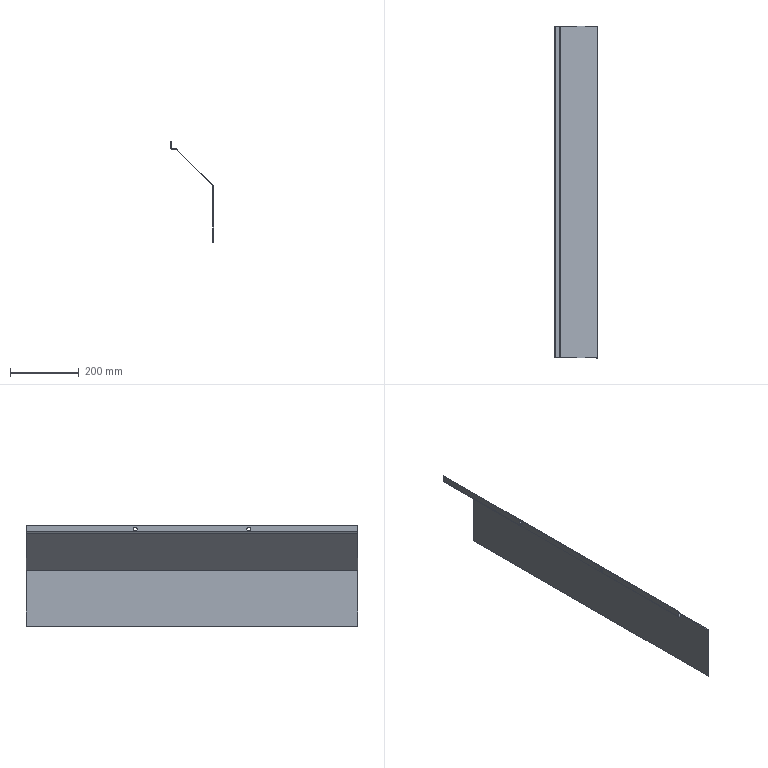Part | STEP file | SYL_0392D6J1SYL0380DJ10-1577336 | 1 solid | 38 faces | box 125 x 964 x 292 mm | volume 507408 mm3 | plane 28 | cylinder 10 | commonest cylinder face diameters 8 x4 4 x3 7 x3
STEP:
#1=CARTESIAN_POINT('',(0.,163.,6.));
#2=VERTEX_POINT('',#1);
#3=CARTESIAN_POINT('',(-1.5,163.,6.));
#4=VERTEX_POINT('',#3);
#5=CARTESIAN_POINT('',(-1.5,163.,6.));
#6=DIRECTION('',(-1.,0.,0.));
#7=VECTOR('',#6,1000.);
#8=LINE('',#5,#7);
#9=EDGE_CURVE('',#2,#4,#8,.T.);
#10=ORIENTED_EDGE('',*,*,#9,.F.);
#11=CARTESIAN_POINT('',(0.,167.,6.));
#12=VERTEX_POINT('',#11);
#13=CARTESIAN_POINT('',(0.,-482.,6.));
#14=DIRECTION('',(0.,1.,0.));
#15=VECTOR('',#14,1000.);
#16=LINE('',#13,#15);
#17=EDGE_CURVE('',#2,#12,#16,.T.);
#18=ORIENTED_EDGE('',*,*,#17,.T.);
#19=CARTESIAN_POINT('',(-1.5,167.,6.));
#20=VERTEX_POINT('',#19);
#21=CARTESIAN_POINT('',(-1.5,167.,6.));
#22=DIRECTION('',(-1.,0.,0.));
#23=VECTOR('',#22,1000.);
#24=LINE('',#21,#23);
#25=EDGE_CURVE('',#12,#20,#24,.T.);
#26=ORIENTED_EDGE('',*,*,#25,.T.);
#27=CARTESIAN_POINT('',(-1.5,163.,6.));
#28=DIRECTION('',(0.,1.,0.));
#29=VECTOR('',#28,1000.);
#30=LINE('',#27,#29);
#31=EDGE_CURVE('',#4,#20,#30,.T.);
#32=ORIENTED_EDGE('',*,*,#31,.F.);
#33=EDGE_LOOP('',(#10,#18,#26,#32));
#34=FACE_OUTER_BOUND('',#33,.T.);
#35=CARTESIAN_POINT('',(-1.5,163.,6.));
#36=DIRECTION('',(0.,0.,-1.));
#37=DIRECTION('',(0.,1.,0.));
#38=AXIS2_PLACEMENT_3D('',#35,#36,#37);
#39=PLANE('',#38);
#40=ADVANCED_FACE('',(#34),#39,.F.);
#41=ORIENTED_EDGE('',*,*,#25,.F.);
#42=CARTESIAN_POINT('',(0.,167.,14.));
#43=VERTEX_POINT('',#42);
#44=CARTESIAN_POINT('',(0.,167.,10.));
#45=DIRECTION('',(1.,0.,0.));
#46=DIRECTION('',(0.,0.,-1.));
#47=AXIS2_PLACEMENT_3D('',#44,#45,#46);
#48=CIRCLE('',#47,4.);
#49=EDGE_CURVE('',#12,#43,#48,.T.);
#50=ORIENTED_EDGE('',*,*,#49,.T.);
#51=CARTESIAN_POINT('',(-1.5,167.,14.));
#52=VERTEX_POINT('',#51);
#53=CARTESIAN_POINT('',(-1.5,167.,14.));
#54=DIRECTION('',(-1.,0.,0.));
#55=VECTOR('',#54,1000.);
#56=LINE('',#53,#55);
#57=EDGE_CURVE('',#43,#52,#56,.T.);
#58=ORIENTED_EDGE('',*,*,#57,.T.);
#59=CARTESIAN_POINT('',(-1.5,167.,10.));
#60=DIRECTION('',(1.,0.,0.));
#61=DIRECTION('',(0.,0.,-1.));
#62=AXIS2_PLACEMENT_3D('',#59,#60,#61);
#63=CIRCLE('',#62,4.);
#64=EDGE_CURVE('',#20,#52,#63,.T.);
#65=ORIENTED_EDGE('',*,*,#64,.F.);
#66=EDGE_LOOP('',(#41,#50,#58,#65));
#67=FACE_OUTER_BOUND('',#66,.T.);
#68=CARTESIAN_POINT('',(-1.5,167.,10.));
#69=DIRECTION('',(1.,0.,0.));
#70=DIRECTION('',(0.,0.,-1.));
#71=AXIS2_PLACEMENT_3D('',#68,#69,#70);
#72=CYLINDRICAL_SURFACE('',#71,4.);
#73=ADVANCED_FACE('',(#67),#72,.F.);
#74=ORIENTED_EDGE('',*,*,#57,.F.);
#75=CARTESIAN_POINT('',(0.,163.,14.));
#76=VERTEX_POINT('',#75);
#77=CARTESIAN_POINT('',(0.,-482.,14.));
#78=DIRECTION('',(0.,-1.,0.));
#79=VECTOR('',#78,1000.);
#80=LINE('',#77,#79);
#81=EDGE_CURVE('',#43,#76,#80,.T.);
#82=ORIENTED_EDGE('',*,*,#81,.T.);
#83=CARTESIAN_POINT('',(-1.5,163.,14.));
#84=VERTEX_POINT('',#83);
#85=CARTESIAN_POINT('',(-1.5,163.,14.));
#86=DIRECTION('',(-1.,0.,0.));
#87=VECTOR('',#86,1000.);
#88=LINE('',#85,#87);
#89=EDGE_CURVE('',#76,#84,#88,.T.);
#90=ORIENTED_EDGE('',*,*,#89,.T.);
#91=CARTESIAN_POINT('',(-1.5,167.,14.));
#92=DIRECTION('',(0.,-1.,0.));
#93=VECTOR('',#92,1000.);
#94=LINE('',#91,#93);
#95=EDGE_CURVE('',#52,#84,#94,.T.);
#96=ORIENTED_EDGE('',*,*,#95,.F.);
#97=EDGE_LOOP('',(#74,#82,#90,#96));
#98=FACE_OUTER_BOUND('',#97,.T.);
#99=CARTESIAN_POINT('',(-1.5,167.,14.));
#100=DIRECTION('',(0.,0.,1.));
#101=DIRECTION('',(0.,-1.,0.));
#102=AXIS2_PLACEMENT_3D('',#99,#100,#101);
#103=PLANE('',#102);
#104=ADVANCED_FACE('',(#98),#103,.F.);
#105=CARTESIAN_POINT('',(0.,-163.,6.));
#106=VERTEX_POINT('',#105);
#107=CARTESIAN_POINT('',(-1.5,-163.,6.));
#108=VERTEX_POINT('',#107);
#109=CARTESIAN_POINT('',(-1.5,-163.,6.));
#110=DIRECTION('',(-1.,0.,0.));
#111=VECTOR('',#110,1000.);
#112=LINE('',#109,#111);
#113=EDGE_CURVE('',#106,#108,#112,.T.);
#114=ORIENTED_EDGE('',*,*,#113,.F.);
#115=CARTESIAN_POINT('',(0.,-163.,14.));
#116=VERTEX_POINT('',#115);
#117=CARTESIAN_POINT('',(0.,-163.,10.));
#118=DIRECTION('',(1.,0.,0.));
#119=DIRECTION('',(0.,0.,-1.));
#120=AXIS2_PLACEMENT_3D('',#117,#118,#119);
#121=CIRCLE('',#120,4.);
#122=EDGE_CURVE('',#106,#116,#121,.T.);
#123=ORIENTED_EDGE('',*,*,#122,.T.);
#124=CARTESIAN_POINT('',(-1.5,-163.,14.));
#125=VERTEX_POINT('',#124);
#126=CARTESIAN_POINT('',(-1.5,-163.,14.));
#127=DIRECTION('',(-1.,0.,0.));
#128=VECTOR('',#127,1000.);
#129=LINE('',#126,#128);
#130=EDGE_CURVE('',#116,#125,#129,.T.);
#131=ORIENTED_EDGE('',*,*,#130,.T.);
#132=CARTESIAN_POINT('',(-1.5,-163.,10.));
#133=DIRECTION('',(1.,0.,0.));
#134=DIRECTION('',(0.,0.,-1.));
#135=AXIS2_PLACEMENT_3D('',#132,#133,#134);
#136=CIRCLE('',#135,4.);
#137=EDGE_CURVE('',#108,#125,#136,.T.);
#138=ORIENTED_EDGE('',*,*,#137,.F.);
#139=EDGE_LOOP('',(#114,#123,#131,#138));
#140=FACE_OUTER_BOUND('',#139,.T.);
#141=CARTESIAN_POINT('',(-1.5,-163.,10.));
#142=DIRECTION('',(1.,0.,0.));
#143=DIRECTION('',(0.,0.,-1.));
#144=AXIS2_PLACEMENT_3D('',#141,#142,#143);
#145=CYLINDRICAL_SURFACE('',#144,4.);
#146=ADVANCED_FACE('',(#140),#145,.F.);
#147=ORIENTED_EDGE('',*,*,#130,.F.);
#148=CARTESIAN_POINT('',(0.,-167.,14.));
#149=VERTEX_POINT('',#148);
#150=CARTESIAN_POINT('',(0.,-482.,14.));
#151=DIRECTION('',(0.,-1.,0.));
#152=VECTOR('',#151,1000.);
#153=LINE('',#150,#152);
#154=EDGE_CURVE('',#116,#149,#153,.T.);
#155=ORIENTED_EDGE('',*,*,#154,.T.);
#156=CARTESIAN_POINT('',(-1.5,-167.,14.));
#157=VERTEX_POINT('',#156);
#158=CARTESIAN_POINT('',(-1.5,-167.,14.));
#159=DIRECTION('',(-1.,0.,0.));
#160=VECTOR('',#159,1000.);
#161=LINE('',#158,#160);
#162=EDGE_CURVE('',#149,#157,#161,.T.);
#163=ORIENTED_EDGE('',*,*,#162,.T.);
#164=CARTESIAN_POINT('',(-1.5,-163.,14.));
#165=DIRECTION('',(0.,-1.,0.));
#166=VECTOR('',#165,1000.);
#167=LINE('',#164,#166);
#168=EDGE_CURVE('',#125,#157,#167,.T.);
#169=ORIENTED_EDGE('',*,*,#168,.F.);
#170=EDGE_LOOP('',(#147,#155,#163,#169));
#171=FACE_OUTER_BOUND('',#170,.T.);
#172=CARTESIAN_POINT('',(-1.5,-163.,14.));
#173=DIRECTION('',(0.,0.,1.));
#174=DIRECTION('',(0.,-1.,0.));
#175=AXIS2_PLACEMENT_3D('',#172,#173,#174);
#176=PLANE('',#175);
#177=ADVANCED_FACE('',(#171),#176,.F.);
#178=ORIENTED_EDGE('',*,*,#162,.F.);
#179=CARTESIAN_POINT('',(0.,-167.,6.));
#180=VERTEX_POINT('',#179);
#181=CARTESIAN_POINT('',(0.,-167.,10.));
#182=DIRECTION('',(1.,0.,0.));
#183=DIRECTION('',(0.,0.,-1.));
#184=AXIS2_PLACEMENT_3D('',#181,#182,#183);
#185=CIRCLE('',#184,4.);
#186=EDGE_CURVE('',#149,#180,#185,.T.);
#187=ORIENTED_EDGE('',*,*,#186,.T.);
#188=CARTESIAN_POINT('',(-1.5,-167.,6.));
#189=VERTEX_POINT('',#188);
#190=CARTESIAN_POINT('',(-1.5,-167.,6.));
#191=DIRECTION('',(-1.,0.,0.));
#192=VECTOR('',#191,1000.);
#193=LINE('',#190,#192);
#194=EDGE_CURVE('',#180,#189,#193,.T.);
#195=ORIENTED_EDGE('',*,*,#194,.T.);
#196=CARTESIAN_POINT('',(-1.5,-167.,10.));
#197=DIRECTION('',(1.,0.,0.));
#198=DIRECTION('',(0.,0.,1.));
#199=AXIS2_PLACEMENT_3D('',#196,#197,#198);
#200=CIRCLE('',#199,4.);
#201=EDGE_CURVE('',#157,#189,#200,.T.);
#202=ORIENTED_EDGE('',*,*,#201,.F.);
#203=EDGE_LOOP('',(#178,#187,#195,#202));
#204=FACE_OUTER_BOUND('',#203,.T.);
#205=CARTESIAN_POINT('',(-1.5,-167.,10.));
#206=DIRECTION('',(1.,0.,0.));
#207=DIRECTION('',(0.,0.,-1.));
#208=AXIS2_PLACEMENT_3D('',#205,#206,#207);
#209=CYLINDRICAL_SURFACE('',#208,4.);
#210=ADVANCED_FACE('',(#204),#209,.F.);
#211=CARTESIAN_POINT('',(0.,-482.,20.));
#212=VERTEX_POINT('',#211);
#213=CARTESIAN_POINT('',(-1.5,-482.,20.));
#214=VERTEX_POINT('',#213);
#215=CARTESIAN_POINT('',(-1.5,-482.,20.));
#216=DIRECTION('',(-1.,0.,0.));
#217=VECTOR('',#216,1000.);
#218=LINE('',#215,#217);
#219=EDGE_CURVE('',#212,#214,#218,.T.);
#220=ORIENTED_EDGE('',*,*,#219,.F.);
#221=CARTESIAN_POINT('',(0.,482.,20.));
#222=VERTEX_POINT('',#221);
#223=CARTESIAN_POINT('',(0.,-482.,20.));
#224=DIRECTION('',(0.,-1.,0.));
#225=VECTOR('',#224,1000.);
#226=LINE('',#223,#225);
#227=EDGE_CURVE('',#222,#212,#226,.T.);
#228=ORIENTED_EDGE('',*,*,#227,.F.);
#229=CARTESIAN_POINT('',(-1.5,482.,20.));
#230=VERTEX_POINT('',#229);
#231=CARTESIAN_POINT('',(-1.5,482.,20.));
#232=DIRECTION('',(-1.,0.,0.));
#233=VECTOR('',#232,1000.);
#234=LINE('',#231,#233);
#235=EDGE_CURVE('',#222,#230,#234,.T.);
#236=ORIENTED_EDGE('',*,*,#235,.T.);
#237=CARTESIAN_POINT('',(-1.5,482.,20.));
#238=DIRECTION('',(0.,-1.,0.));
#239=VECTOR('',#238,1000.);
#240=LINE('',#237,#239);
#241=EDGE_CURVE('',#230,#214,#240,.T.);
#242=ORIENTED_EDGE('',*,*,#241,.T.);
#243=EDGE_LOOP('',(#220,#228,#236,#242));
#244=FACE_OUTER_BOUND('',#243,.T.);
#245=CARTESIAN_POINT('',(-1.5,482.,20.));
#246=DIRECTION('',(0.,0.,1.));
#247=DIRECTION('',(0.,-1.,0.));
#248=AXIS2_PLACEMENT_3D('',#245,#246,#247);
#249=PLANE('',#248);
#250=ADVANCED_FACE('',(#244),#249,.T.);
#251=ORIENTED_EDGE('',*,*,#235,.F.);
#252=CARTESIAN_POINT('',(0.,482.,2.));
#253=VERTEX_POINT('',#252);
#254=CARTESIAN_POINT('',(0.,482.,20.));
#255=DIRECTION('',(0.,0.,1.));
#256=VECTOR('',#255,1000.);
#257=LINE('',#254,#256);
#258=EDGE_CURVE('',#253,#222,#257,.T.);
#259=ORIENTED_EDGE('',*,*,#258,.F.);
#260=CARTESIAN_POINT('',(-1.5,482.,2.));
#261=VERTEX_POINT('',#260);
#262=CARTESIAN_POINT('',(-1.5,482.,2.));
#263=DIRECTION('',(-1.,0.,0.));
#264=VECTOR('',#263,1000.);
#265=LINE('',#262,#264);
#266=EDGE_CURVE('',#253,#261,#265,.T.);
#267=ORIENTED_EDGE('',*,*,#266,.T.);
#268=CARTESIAN_POINT('',(-1.5,482.,2.));
#269=DIRECTION('',(0.,0.,1.));
#270=VECTOR('',#269,1000.);
#271=LINE('',#268,#270);
#272=EDGE_CURVE('',#261,#230,#271,.T.);
#273=ORIENTED_EDGE('',*,*,#272,.T.);
#274=EDGE_LOOP('',(#251,#259,#267,#273));
#275=FACE_OUTER_BOUND('',#274,.T.);
#276=CARTESIAN_POINT('',(-1.5,482.,2.));
#277=DIRECTION('',(0.,1.,0.));
#278=DIRECTION('',(0.,0.,1.));
#279=AXIS2_PLACEMENT_3D('',#276,#277,#278);
#280=PLANE('',#279);
#281=ADVANCED_FACE('',(#275),#280,.T.);
#282=ORIENTED_EDGE('',*,*,#266,.F.);
#283=CARTESIAN_POINT('',(2.,482.,0.));
#284=VERTEX_POINT('',#283);
#285=CARTESIAN_POINT('',(2.,482.,2.));
#286=DIRECTION('',(0.,1.,0.));
#287=DIRECTION('',(0.,0.,1.));
#288=AXIS2_PLACEMENT_3D('',#285,#286,#287);
#289=CIRCLE('',#288,2.);
#290=EDGE_CURVE('',#284,#253,#289,.T.);
#291=ORIENTED_EDGE('',*,*,#290,.F.);
#292=CARTESIAN_POINT('',(2.,482.,-1.5));
#293=VERTEX_POINT('',#292);
#294=CARTESIAN_POINT('',(2.,482.,-1.5));
#295=DIRECTION('',(0.,0.,-1.));
#296=VECTOR('',#295,1000.);
#297=LINE('',#294,#296);
#298=EDGE_CURVE('',#284,#293,#297,.T.);
#299=ORIENTED_EDGE('',*,*,#298,.T.);
#300=CARTESIAN_POINT('',(2.,482.,2.));
#301=DIRECTION('',(0.,1.,0.));
#302=DIRECTION('',(0.,0.,-1.));
#303=AXIS2_PLACEMENT_3D('',#300,#301,#302);
#304=CIRCLE('',#303,3.5);
#305=EDGE_CURVE('',#293,#261,#304,.T.);
#306=ORIENTED_EDGE('',*,*,#305,.T.);
#307=EDGE_LOOP('',(#282,#291,#299,#306));
#308=FACE_OUTER_BOUND('',#307,.T.);
#309=CARTESIAN_POINT('',(2.,482.,2.));
#310=DIRECTION('',(0.,-1.,0.));
#311=DIRECTION('',(0.,0.,-1.));
#312=AXIS2_PLACEMENT_3D('',#309,#310,#311);
#313=PLANE('',#312);
#314=ADVANCED_FACE('',(#308),#313,.F.);
#315=ORIENTED_EDGE('',*,*,#298,.F.);
#316=CARTESIAN_POINT('',(14.05,482.,0.));
#317=VERTEX_POINT('',#316);
#318=CARTESIAN_POINT('',(0.,482.,0.));
#319=DIRECTION('',(-1.,0.,0.));
#320=VECTOR('',#319,1000.);
#321=LINE('',#318,#320);
#322=EDGE_CURVE('',#317,#284,#321,.T.);
#323=ORIENTED_EDGE('',*,*,#322,.F.);
#324=CARTESIAN_POINT('',(14.05,482.,-1.5));
#325=VERTEX_POINT('',#324);
#326=CARTESIAN_POINT('',(14.05,482.,-1.5));
#327=DIRECTION('',(0.,0.,-1.));
#328=VECTOR('',#327,1000.);
#329=LINE('',#326,#328);
#330=EDGE_CURVE('',#317,#325,#329,.T.);
#331=ORIENTED_EDGE('',*,*,#330,.T.);
#332=CARTESIAN_POINT('',(14.05,482.,-1.5));
#333=DIRECTION('',(-1.,0.,0.));
#334=VECTOR('',#333,1000.);
#335=LINE('',#332,#334);
#336=EDGE_CURVE('',#325,#293,#335,.T.);
#337=ORIENTED_EDGE('',*,*,#336,.T.);
#338=EDGE_LOOP('',(#315,#323,#331,#337));
#339=FACE_OUTER_BOUND('',#338,.T.);
#340=CARTESIAN_POINT('',(14.05,482.,-1.5));
#341=DIRECTION('',(0.,1.,0.));
#342=DIRECTION('',(-1.,0.,0.));
#343=AXIS2_PLACEMENT_3D('',#340,#341,#342);
#344=PLANE('',#343);
#345=ADVANCED_FACE('',(#339),#344,.T.);
#346=ORIENTED_EDGE('',*,*,#330,.F.);
#347=CARTESIAN_POINT('',(16.525,482.,-1.025));
#348=VERTEX_POINT('',#347);
#349=CARTESIAN_POINT('',(14.05,482.,-3.5));
#350=DIRECTION('',(0.,-1.,0.));
#351=DIRECTION('',(0.,0.,-1.));
#352=AXIS2_PLACEMENT_3D('',#349,#350,#351);
#353=CIRCLE('',#352,3.5);
#354=EDGE_CURVE('',#348,#317,#353,.T.);
#355=ORIENTED_EDGE('',*,*,#354,.F.);
#356=CARTESIAN_POINT('',(15.464,482.,-2.086));
#357=VERTEX_POINT('',#356);
#358=CARTESIAN_POINT('',(15.464,482.,-2.086));
#359=DIRECTION('',(-0.7071,0.,-0.7071));
#360=VECTOR('',#359,1000.);
#361=LINE('',#358,#360);
#362=EDGE_CURVE('',#348,#357,#361,.T.);
#363=ORIENTED_EDGE('',*,*,#362,.T.);
#364=CARTESIAN_POINT('',(14.05,482.,-3.5));
#365=DIRECTION('',(0.,-1.,0.));
#366=DIRECTION('',(0.7071,0.,0.7071));
#367=AXIS2_PLACEMENT_3D('',#364,#365,#366);
#368=CIRCLE('',#367,2.);
#369=EDGE_CURVE('',#357,#325,#368,.T.);
#370=ORIENTED_EDGE('',*,*,#369,.T.);
#371=EDGE_LOOP('',(#346,#355,#363,#370));
#372=FACE_OUTER_BOUND('',#371,.T.);
#373=CARTESIAN_POINT('',(14.05,482.,-3.5));
#374=DIRECTION('',(0.,1.,0.));
#375=DIRECTION('',(0.,0.,1.));
#376=AXIS2_PLACEMENT_3D('',#373,#374,#375);
#377=PLANE('',#376);
#378=ADVANCED_FACE('',(#372),#377,.T.);
#379=ORIENTED_EDGE('',*,*,#362,.F.);
#380=CARTESIAN_POINT('',(122.475,482.,-106.975));
#381=VERTEX_POINT('',#380);
#382=CARTESIAN_POINT('',(15.5,482.,0.));
#383=DIRECTION('',(-0.7071,0.,0.7071));
#384=VECTOR('',#383,1000.);
#385=LINE('',#382,#384);
#386=EDGE_CURVE('',#381,#348,#385,.T.);
#387=ORIENTED_EDGE('',*,*,#386,.F.);
#388=CARTESIAN_POINT('',(121.414,482.,-108.036));
#389=VERTEX_POINT('',#388);
#390=CARTESIAN_POINT('',(121.414,482.,-108.036));
#391=DIRECTION('',(-0.7071,0.,-0.7071));
#392=VECTOR('',#391,1000.);
#393=LINE('',#390,#392);
#394=EDGE_CURVE('',#381,#389,#393,.T.);
#395=ORIENTED_EDGE('',*,*,#394,.T.);
#396=CARTESIAN_POINT('',(121.414,482.,-108.036));
#397=DIRECTION('',(-0.7071,0.,0.7071));
#398=VECTOR('',#397,1000.);
#399=LINE('',#396,#398);
#400=EDGE_CURVE('',#389,#357,#399,.T.);
#401=ORIENTED_EDGE('',*,*,#400,.T.);
#402=EDGE_LOOP('',(#379,#387,#395,#401));
#403=FACE_OUTER_BOUND('',#402,.T.);
#404=CARTESIAN_POINT('',(121.414,482.,-108.036));
#405=DIRECTION('',(0.,1.,0.));
#406=DIRECTION('',(-0.7071,0.,0.7071));
#407=AXIS2_PLACEMENT_3D('',#404,#405,#406);
#408=PLANE('',#407);
#409=ADVANCED_FACE('',(#403),#408,.T.);
#410=ORIENTED_EDGE('',*,*,#394,.F.);
#411=CARTESIAN_POINT('',(123.5,482.,-109.45));
#412=VERTEX_POINT('',#411);
#413=CARTESIAN_POINT('',(120.,482.,-109.45));
#414=DIRECTION('',(0.,-1.,0.));
#415=DIRECTION('',(0.,0.,-1.));
#416=AXIS2_PLACEMENT_3D('',#413,#414,#415);
#417=CIRCLE('',#416,3.5);
#418=EDGE_CURVE('',#412,#381,#417,.T.);
#419=ORIENTED_EDGE('',*,*,#418,.F.);
#420=CARTESIAN_POINT('',(122.,482.,-109.45));
#421=VERTEX_POINT('',#420);
#422=CARTESIAN_POINT('',(122.,482.,-109.45));
#423=DIRECTION('',(-1.,0.,0.));
#424=VECTOR('',#423,1000.);
#425=LINE('',#422,#424);
#426=EDGE_CURVE('',#412,#421,#425,.T.);
#427=ORIENTED_EDGE('',*,*,#426,.T.);
#428=CARTESIAN_POINT('',(120.,482.,-109.45));
#429=DIRECTION('',(0.,-1.,0.));
#430=DIRECTION('',(1.,0.,0.));
#431=AXIS2_PLACEMENT_3D('',#428,#429,#430);
#432=CIRCLE('',#431,2.);
#433=EDGE_CURVE('',#421,#389,#432,.T.);
#434=ORIENTED_EDGE('',*,*,#433,.T.);
#435=EDGE_LOOP('',(#410,#419,#427,#434));
#436=FACE_OUTER_BOUND('',#435,.T.);
#437=CARTESIAN_POINT('',(120.,482.,-109.45));
#438=DIRECTION('',(0.,1.,0.));
#439=DIRECTION('',(0.,0.,1.));
#440=AXIS2_PLACEMENT_3D('',#437,#438,#439);
#441=PLANE('',#440);
#442=ADVANCED_FACE('',(#436),#441,.T.);
#443=ORIENTED_EDGE('',*,*,#426,.F.);
#444=CARTESIAN_POINT('',(123.5,482.,-272.));
#445=VERTEX_POINT('',#444);
#446=CARTESIAN_POINT('',(123.5,482.,-108.));
#447=DIRECTION('',(0.,0.,1.));
#448=VECTOR('',#447,1000.);
#449=LINE('',#446,#448);
#450=EDGE_CURVE('',#445,#412,#449,.T.);
#451=ORIENTED_EDGE('',*,*,#450,.F.);
#452=CARTESIAN_POINT('',(122.,482.,-272.));
#453=VERTEX_POINT('',#452);
#454=CARTESIAN_POINT('',(122.,482.,-272.));
#455=DIRECTION('',(-1.,0.,0.));
#456=VECTOR('',#455,1000.);
#457=LINE('',#454,#456);
#458=EDGE_CURVE('',#445,#453,#457,.T.);
#459=ORIENTED_EDGE('',*,*,#458,.T.);
#460=CARTESIAN_POINT('',(122.,482.,-272.));
#461=DIRECTION('',(0.,0.,1.));
#462=VECTOR('',#461,1000.);
#463=LINE('',#460,#462);
#464=EDGE_CURVE('',#453,#421,#463,.T.);
#465=ORIENTED_EDGE('',*,*,#464,.T.);
#466=EDGE_LOOP('',(#443,#451,#459,#465));
#467=FACE_OUTER_BOUND('',#466,.T.);
#468=CARTESIAN_POINT('',(122.,482.,-272.));
#469=DIRECTION('',(0.,1.,0.));
#470=DIRECTION('',(0.,0.,1.));
#471=AXIS2_PLACEMENT_3D('',#468,#469,#470);
#472=PLANE('',#471);
#473=ADVANCED_FACE('',(#467),#472,.T.);
#474=ORIENTED_EDGE('',*,*,#458,.F.);
#475=CARTESIAN_POINT('',(123.5,-482.,-272.));
#476=VERTEX_POINT('',#475);
#477=CARTESIAN_POINT('',(123.5,-482.,-272.));
#478=DIRECTION('',(0.,-1.,0.));
#479=VECTOR('',#478,1000.);
#480=LINE('',#477,#479);
#481=EDGE_CURVE('',#445,#476,#480,.T.);
#482=ORIENTED_EDGE('',*,*,#481,.T.);
#483=CARTESIAN_POINT('',(122.,-482.,-272.));
#484=VERTEX_POINT('',#483);
#485=CARTESIAN_POINT('',(122.,-482.,-272.));
#486=DIRECTION('',(-1.,0.,0.));
#487=VECTOR('',#486,1000.);
#488=LINE('',#485,#487);
#489=EDGE_CURVE('',#476,#484,#488,.T.);
#490=ORIENTED_EDGE('',*,*,#489,.T.);
#491=CARTESIAN_POINT('',(122.,482.,-272.));
#492=DIRECTION('',(0.,-1.,0.));
#493=VECTOR('',#492,1000.);
#494=LINE('',#491,#493);
#495=EDGE_CURVE('',#453,#484,#494,.T.);
#496=ORIENTED_EDGE('',*,*,#495,.F.);
#497=EDGE_LOOP('',(#474,#482,#490,#496));
#498=FACE_OUTER_BOUND('',#497,.T.);
#499=CARTESIAN_POINT('',(122.,482.,-272.));
#500=DIRECTION('',(0.,0.,1.));
#501=DIRECTION('',(0.,-1.,0.));
#502=AXIS2_PLACEMENT_3D('',#499,#500,#501);
#503=PLANE('',#502);
#504=ADVANCED_FACE('',(#498),#503,.F.);
#505=ORIENTED_EDGE('',*,*,#489,.F.);
#506=CARTESIAN_POINT('',(123.5,-482.,-109.45));
#507=VERTEX_POINT('',#506);
#508=CARTESIAN_POINT('',(123.5,-482.,-108.));
#509=DIRECTION('',(0.,0.,1.));
#510=VECTOR('',#509,1000.);
#511=LINE('',#508,#510);
#512=EDGE_CURVE('',#476,#507,#511,.T.);
#513=ORIENTED_EDGE('',*,*,#512,.T.);
#514=CARTESIAN_POINT('',(122.,-482.,-109.45));
#515=VERTEX_POINT('',#514);
#516=CARTESIAN_POINT('',(122.,-482.,-109.45));
#517=DIRECTION('',(-1.,0.,0.));
#518=VECTOR('',#517,1000.);
#519=LINE('',#516,#518);
#520=EDGE_CURVE('',#507,#515,#519,.T.);
#521=ORIENTED_EDGE('',*,*,#520,.T.);
#522=CARTESIAN_POINT('',(122.,-482.,-272.));
#523=DIRECTION('',(0.,0.,1.));
#524=VECTOR('',#523,1000.);
#525=LINE('',#522,#524);
#526=EDGE_CURVE('',#484,#515,#525,.T.);
#527=ORIENTED_EDGE('',*,*,#526,.F.);
#528=EDGE_LOOP('',(#505,#513,#521,#527));
#529=FACE_OUTER_BOUND('',#528,.T.);
#530=CARTESIAN_POINT('',(122.,-482.,-272.));
#531=DIRECTION('',(0.,1.,0.));
#532=DIRECTION('',(0.,0.,1.));
#533=AXIS2_PLACEMENT_3D('',#530,#531,#532);
#534=PLANE('',#533);
#535=ADVANCED_FACE('',(#529),#534,.F.);
#536=ORIENTED_EDGE('',*,*,#520,.F.);
#537=CARTESIAN_POINT('',(122.475,-482.,-106.975));
#538=VERTEX_POINT('',#537);
#539=CARTESIAN_POINT('',(120.,-482.,-109.45));
#540=DIRECTION('',(0.,1.,0.));
#541=DIRECTION('',(0.,0.,-1.));
#542=AXIS2_PLACEMENT_3D('',#539,#540,#541);
#543=CIRCLE('',#542,3.5);
#544=EDGE_CURVE('',#538,#507,#543,.T.);
#545=ORIENTED_EDGE('',*,*,#544,.F.);
#546=CARTESIAN_POINT('',(121.414,-482.,-108.036));
#547=VERTEX_POINT('',#546);
#548=CARTESIAN_POINT('',(121.414,-482.,-108.036));
#549=DIRECTION('',(-0.7071,0.,-0.7071));
#550=VECTOR('',#549,1000.);
#551=LINE('',#548,#550);
#552=EDGE_CURVE('',#538,#547,#551,.T.);
#553=ORIENTED_EDGE('',*,*,#552,.T.);
#554=CARTESIAN_POINT('',(120.,-482.,-109.45));
#555=DIRECTION('',(0.,1.,0.));
#556=DIRECTION('',(0.7071,0.,0.7071));
#557=AXIS2_PLACEMENT_3D('',#554,#555,#556);
#558=CIRCLE('',#557,2.);
#559=EDGE_CURVE('',#547,#515,#558,.T.);
#560=ORIENTED_EDGE('',*,*,#559,.T.);
#561=EDGE_LOOP('',(#536,#545,#553,#560));
#562=FACE_OUTER_BOUND('',#561,.T.);
#563=CARTESIAN_POINT('',(120.,-482.,-109.45));
#564=DIRECTION('',(0.,-1.,0.));
#565=DIRECTION('',(0.,0.,-1.));
#566=AXIS2_PLACEMENT_3D('',#563,#564,#565);
#567=PLANE('',#566);
#568=ADVANCED_FACE('',(#562),#567,.T.);
#569=ORIENTED_EDGE('',*,*,#552,.F.);
#570=CARTESIAN_POINT('',(16.525,-482.,-1.025));
#571=VERTEX_POINT('',#570);
#572=CARTESIAN_POINT('',(15.5,-482.,0.));
#573=DIRECTION('',(0.7071,0.,-0.7071));
#574=VECTOR('',#573,1000.);
#575=LINE('',#572,#574);
#576=EDGE_CURVE('',#571,#538,#575,.T.);
#577=ORIENTED_EDGE('',*,*,#576,.F.);
#578=CARTESIAN_POINT('',(15.464,-482.,-2.086));
#579=VERTEX_POINT('',#578);
#580=CARTESIAN_POINT('',(15.464,-482.,-2.086));
#581=DIRECTION('',(-0.7071,0.,-0.7071));
#582=VECTOR('',#581,1000.);
#583=LINE('',#580,#582);
#584=EDGE_CURVE('',#571,#579,#583,.T.);
#585=ORIENTED_EDGE('',*,*,#584,.T.);
#586=CARTESIAN_POINT('',(15.464,-482.,-2.086));
#587=DIRECTION('',(0.7071,0.,-0.7071));
#588=VECTOR('',#587,1000.);
#589=LINE('',#586,#588);
#590=EDGE_CURVE('',#579,#547,#589,.T.);
#591=ORIENTED_EDGE('',*,*,#590,.T.);
#592=EDGE_LOOP('',(#569,#577,#585,#591));
#593=FACE_OUTER_BOUND('',#592,.T.);
#594=CARTESIAN_POINT('',(15.464,-482.,-2.086));
#595=DIRECTION('',(0.,-1.,0.));
#596=DIRECTION('',(0.7071,0.,-0.7071));
#597=AXIS2_PLACEMENT_3D('',#594,#595,#596);
#598=PLANE('',#597);
#599=ADVANCED_FACE('',(#593),#598,.T.);
#600=ORIENTED_EDGE('',*,*,#584,.F.);
#601=CARTESIAN_POINT('',(14.05,-482.,0.));
#602=VERTEX_POINT('',#601);
#603=CARTESIAN_POINT('',(14.05,-482.,-3.5));
#604=DIRECTION('',(0.,1.,0.));
#605=DIRECTION('',(0.,0.,-1.));
#606=AXIS2_PLACEMENT_3D('',#603,#604,#605);
#607=CIRCLE('',#606,3.5);
#608=EDGE_CURVE('',#602,#571,#607,.T.);
#609=ORIENTED_EDGE('',*,*,#608,.F.);
#610=CARTESIAN_POINT('',(14.05,-482.,-1.5));
#611=VERTEX_POINT('',#610);
#612=CARTESIAN_POINT('',(14.05,-482.,-1.5));
#613=DIRECTION('',(0.,0.,-1.));
#614=VECTOR('',#613,1000.);
#615=LINE('',#612,#614);
#616=EDGE_CURVE('',#602,#611,#615,.T.);
#617=ORIENTED_EDGE('',*,*,#616,.T.);
#618=CARTESIAN_POINT('',(14.05,-482.,-3.5));
#619=DIRECTION('',(0.,1.,0.));
#620=DIRECTION('',(0.,0.,1.));
#621=AXIS2_PLACEMENT_3D('',#618,#619,#620);
#622=CIRCLE('',#621,2.);
#623=EDGE_CURVE('',#611,#579,#622,.T.);
#624=ORIENTED_EDGE('',*,*,#623,.T.);
#625=EDGE_LOOP('',(#600,#609,#617,#624));
#626=FACE_OUTER_BOUND('',#625,.T.);
#627=CARTESIAN_POINT('',(14.05,-482.,-3.5));
#628=DIRECTION('',(0.,-1.,0.));
#629=DIRECTION('',(0.,0.,-1.));
#630=AXIS2_PLACEMENT_3D('',#627,#628,#629);
#631=PLANE('',#630);
#632=ADVANCED_FACE('',(#626),#631,.T.);
#633=ORIENTED_EDGE('',*,*,#616,.F.);
#634=CARTESIAN_POINT('',(2.,-482.,0.));
#635=VERTEX_POINT('',#634);
#636=CARTESIAN_POINT('',(0.,-482.,0.));
#637=DIRECTION('',(-1.,0.,0.));
#638=VECTOR('',#637,1000.);
#639=LINE('',#636,#638);
#640=EDGE_CURVE('',#602,#635,#639,.T.);
#641=ORIENTED_EDGE('',*,*,#640,.T.);
#642=CARTESIAN_POINT('',(2.,-482.,-1.5));
#643=VERTEX_POINT('',#642);
#644=CARTESIAN_POINT('',(2.,-482.,-1.5));
#645=DIRECTION('',(0.,0.,-1.));
#646=VECTOR('',#645,1000.);
#647=LINE('',#644,#646);
#648=EDGE_CURVE('',#635,#643,#647,.T.);
#649=ORIENTED_EDGE('',*,*,#648,.T.);
#650=CARTESIAN_POINT('',(14.05,-482.,-1.5));
#651=DIRECTION('',(-1.,0.,0.));
#652=VECTOR('',#651,1000.);
#653=LINE('',#650,#652);
#654=EDGE_CURVE('',#611,#643,#653,.T.);
#655=ORIENTED_EDGE('',*,*,#654,.F.);
#656=EDGE_LOOP('',(#633,#641,#649,#655));
#657=FACE_OUTER_BOUND('',#656,.T.);
#658=CARTESIAN_POINT('',(14.05,-482.,-1.5));
#659=DIRECTION('',(0.,1.,0.));
#660=DIRECTION('',(-1.,0.,0.));
#661=AXIS2_PLACEMENT_3D('',#658,#659,#660);
#662=PLANE('',#661);
#663=ADVANCED_FACE('',(#657),#662,.F.);
#664=ORIENTED_EDGE('',*,*,#648,.F.);
#665=CARTESIAN_POINT('',(0.,-482.,2.));
#666=VERTEX_POINT('',#665);
#667=CARTESIAN_POINT('',(2.,-482.,2.));
#668=DIRECTION('',(0.,-1.,0.));
#669=DIRECTION('',(0.,0.,1.));
#670=AXIS2_PLACEMENT_3D('',#667,#668,#669);
#671=CIRCLE('',#670,2.);
#672=EDGE_CURVE('',#666,#635,#671,.T.);
#673=ORIENTED_EDGE('',*,*,#672,.F.);
#674=CARTESIAN_POINT('',(-1.5,-482.,2.));
#675=VERTEX_POINT('',#674);
#676=CARTESIAN_POINT('',(-1.5,-482.,2.));
#677=DIRECTION('',(-1.,0.,0.));
#678=VECTOR('',#677,1000.);
#679=LINE('',#676,#678);
#680=EDGE_CURVE('',#666,#675,#679,.T.);
#681=ORIENTED_EDGE('',*,*,#680,.T.);
#682=CARTESIAN_POINT('',(2.,-482.,2.));
#683=DIRECTION('',(0.,-1.,0.));
#684=DIRECTION('',(-1.,0.,0.));
#685=AXIS2_PLACEMENT_3D('',#682,#683,#684);
#686=CIRCLE('',#685,3.5);
#687=EDGE_CURVE('',#675,#643,#686,.T.);
#688=ORIENTED_EDGE('',*,*,#687,.T.);
#689=EDGE_LOOP('',(#664,#673,#681,#688));
#690=FACE_OUTER_BOUND('',#689,.T.);
#691=CARTESIAN_POINT('',(2.,-482.,2.));
#692=DIRECTION('',(0.,1.,0.));
#693=DIRECTION('',(0.,0.,1.));
#694=AXIS2_PLACEMENT_3D('',#691,#692,#693);
#695=PLANE('',#694);
#696=ADVANCED_FACE('',(#690),#695,.F.);
#697=CARTESIAN_POINT('',(0.,-482.,6.));
#698=DIRECTION('',(0.,1.,0.));
#699=VECTOR('',#698,1000.);
#700=LINE('',#697,#699);
#701=EDGE_CURVE('',#180,#106,#700,.T.);
#702=ORIENTED_EDGE('',*,*,#701,.T.);
#703=ORIENTED_EDGE('',*,*,#113,.T.);
#704=CARTESIAN_POINT('',(-1.5,-167.,6.));
#705=DIRECTION('',(0.,1.,0.));
#706=VECTOR('',#705,1000.);
#707=LINE('',#704,#706);
#708=EDGE_CURVE('',#189,#108,#707,.T.);
#709=ORIENTED_EDGE('',*,*,#708,.F.);
#710=ORIENTED_EDGE('',*,*,#194,.F.);
#711=EDGE_LOOP('',(#702,#703,#709,#710));
#712=FACE_OUTER_BOUND('',#711,.T.);
#713=CARTESIAN_POINT('',(-1.5,-167.,6.));
#714=DIRECTION('',(0.,0.,-1.));
#715=DIRECTION('',(0.,1.,0.));
#716=AXIS2_PLACEMENT_3D('',#713,#714,#715);
#717=PLANE('',#716);
#718=ADVANCED_FACE('',(#712),#717,.F.);
#719=CARTESIAN_POINT('',(0.,163.,10.));
#720=DIRECTION('',(1.,0.,0.));
#721=DIRECTION('',(0.,0.,-1.));
#722=AXIS2_PLACEMENT_3D('',#719,#720,#721);
#723=CIRCLE('',#722,4.);
#724=EDGE_CURVE('',#76,#2,#723,.T.);
#725=ORIENTED_EDGE('',*,*,#724,.T.);
#726=ORIENTED_EDGE('',*,*,#9,.T.);
#727=CARTESIAN_POINT('',(-1.5,163.,10.));
#728=DIRECTION('',(1.,0.,0.));
#729=DIRECTION('',(0.,0.,1.));
#730=AXIS2_PLACEMENT_3D('',#727,#728,#729);
#731=CIRCLE('',#730,4.);
#732=EDGE_CURVE('',#84,#4,#731,.T.);
#733=ORIENTED_EDGE('',*,*,#732,.F.);
#734=ORIENTED_EDGE('',*,*,#89,.F.);
#735=EDGE_LOOP('',(#725,#726,#733,#734));
#736=FACE_OUTER_BOUND('',#735,.T.);
#737=CARTESIAN_POINT('',(-1.5,163.,10.));
#738=DIRECTION('',(1.,0.,0.));
#739=DIRECTION('',(0.,0.,-1.));
#740=AXIS2_PLACEMENT_3D('',#737,#738,#739);
#741=CYLINDRICAL_SURFACE('',#740,4.);
#742=ADVANCED_FACE('',(#736),#741,.F.);
#743=CARTESIAN_POINT('',(0.,-482.,20.));
#744=DIRECTION('',(0.,0.,1.));
#745=VECTOR('',#744,1000.);
#746=LINE('',#743,#745);
#747=EDGE_CURVE('',#666,#212,#746,.T.);
#748=ORIENTED_EDGE('',*,*,#747,.T.);
#749=ORIENTED_EDGE('',*,*,#219,.T.);
#750=CARTESIAN_POINT('',(-1.5,-482.,2.));
#751=DIRECTION('',(0.,0.,1.));
#752=VECTOR('',#751,1000.);
#753=LINE('',#750,#752);
#754=EDGE_CURVE('',#675,#214,#753,.T.);
#755=ORIENTED_EDGE('',*,*,#754,.F.);
#756=ORIENTED_EDGE('',*,*,#680,.F.);
#757=EDGE_LOOP('',(#748,#749,#755,#756));
#758=FACE_OUTER_BOUND('',#757,.T.);
#759=CARTESIAN_POINT('',(-1.5,-482.,2.));
#760=DIRECTION('',(0.,1.,0.));
#761=DIRECTION('',(0.,0.,1.));
#762=AXIS2_PLACEMENT_3D('',#759,#760,#761);
#763=PLANE('',#762);
#764=ADVANCED_FACE('',(#758),#763,.F.);
#765=CARTESIAN_POINT('',(2.,482.,-1.5));
#766=DIRECTION('',(0.,-1.,0.));
#767=VECTOR('',#766,1000.);
#768=LINE('',#765,#767);
#769=EDGE_CURVE('',#293,#643,#768,.T.);
#770=ORIENTED_EDGE('',*,*,#769,.T.);
#771=ORIENTED_EDGE('',*,*,#687,.F.);
#772=CARTESIAN_POINT('',(-1.5,-482.,2.));
#773=DIRECTION('',(0.,1.,0.));
#774=VECTOR('',#773,1000.);
#775=LINE('',#772,#774);
#776=EDGE_CURVE('',#675,#261,#775,.T.);
#777=ORIENTED_EDGE('',*,*,#776,.T.);
#778=ORIENTED_EDGE('',*,*,#305,.F.);
#779=EDGE_LOOP('',(#770,#771,#777,#778));
#780=FACE_OUTER_BOUND('',#779,.T.);
#781=CARTESIAN_POINT('',(2.,-482.,2.));
#782=DIRECTION('',(0.,1.,0.));
#783=DIRECTION('',(0.,0.,1.));
#784=AXIS2_PLACEMENT_3D('',#781,#782,#783);
#785=CYLINDRICAL_SURFACE('',#784,3.5);
#786=ADVANCED_FACE('',(#780),#785,.T.);
#787=ORIENTED_EDGE('',*,*,#201,.T.);
#788=ORIENTED_EDGE('',*,*,#708,.T.);
#789=ORIENTED_EDGE('',*,*,#137,.T.);
#790=ORIENTED_EDGE('',*,*,#168,.T.);
#791=EDGE_LOOP('',(#787,#788,#789,#790));
#792=FACE_BOUND('',#791,.T.);
#793=ORIENTED_EDGE('',*,*,#95,.T.);
#794=ORIENTED_EDGE('',*,*,#732,.T.);
#795=ORIENTED_EDGE('',*,*,#31,.T.);
#796=ORIENTED_EDGE('',*,*,#64,.T.);
#797=EDGE_LOOP('',(#793,#794,#795,#796));
#798=FACE_BOUND('',#797,.T.);
#799=ORIENTED_EDGE('',*,*,#776,.F.);
#800=ORIENTED_EDGE('',*,*,#754,.T.);
#801=ORIENTED_EDGE('',*,*,#241,.F.);
#802=ORIENTED_EDGE('',*,*,#272,.F.);
#803=EDGE_LOOP('',(#799,#800,#801,#802));
#804=FACE_OUTER_BOUND('',#803,.T.);
#805=CARTESIAN_POINT('',(-1.5,-482.,20.));
#806=DIRECTION('',(1.,0.,0.));
#807=DIRECTION('',(0.,1.,0.));
#808=AXIS2_PLACEMENT_3D('',#805,#806,#807);
#809=PLANE('',#808);
#810=ADVANCED_FACE('',(#792,#798,#804),#809,.F.);
#811=ORIENTED_EDGE('',*,*,#369,.F.);
#812=CARTESIAN_POINT('',(15.464,482.,-2.086));
#813=DIRECTION('',(0.,-1.,0.));
#814=VECTOR('',#813,1000.);
#815=LINE('',#812,#814);
#816=EDGE_CURVE('',#357,#579,#815,.T.);
#817=ORIENTED_EDGE('',*,*,#816,.T.);
#818=ORIENTED_EDGE('',*,*,#623,.F.);
#819=CARTESIAN_POINT('',(14.05,-482.,-1.5));
#820=DIRECTION('',(0.,1.,0.));
#821=VECTOR('',#820,1000.);
#822=LINE('',#819,#821);
#823=EDGE_CURVE('',#611,#325,#822,.T.);
#824=ORIENTED_EDGE('',*,*,#823,.T.);
#825=EDGE_LOOP('',(#811,#817,#818,#824));
#826=FACE_OUTER_BOUND('',#825,.T.);
#827=CARTESIAN_POINT('',(14.05,-482.,-3.5));
#828=DIRECTION('',(0.,-1.,0.));
#829=DIRECTION('',(0.,0.,-1.));
#830=AXIS2_PLACEMENT_3D('',#827,#828,#829);
#831=CYLINDRICAL_SURFACE('',#830,2.);
#832=ADVANCED_FACE('',(#826),#831,.F.);
#833=ORIENTED_EDGE('',*,*,#823,.F.);
#834=ORIENTED_EDGE('',*,*,#654,.T.);
#835=ORIENTED_EDGE('',*,*,#769,.F.);
#836=ORIENTED_EDGE('',*,*,#336,.F.);
#837=EDGE_LOOP('',(#833,#834,#835,#836));
#838=FACE_OUTER_BOUND('',#837,.T.);
#839=CARTESIAN_POINT('',(0.,-482.,-1.5));
#840=DIRECTION('',(0.,0.,1.));
#841=DIRECTION('',(1.,0.,0.));
#842=AXIS2_PLACEMENT_3D('',#839,#840,#841);
#843=PLANE('',#842);
#844=ADVANCED_FACE('',(#838),#843,.F.);
#845=ORIENTED_EDGE('',*,*,#433,.F.);
#846=CARTESIAN_POINT('',(122.,482.,-109.45));
#847=DIRECTION('',(0.,-1.,0.));
#848=VECTOR('',#847,1000.);
#849=LINE('',#846,#848);
#850=EDGE_CURVE('',#421,#515,#849,.T.);
#851=ORIENTED_EDGE('',*,*,#850,.T.);
#852=ORIENTED_EDGE('',*,*,#559,.F.);
#853=CARTESIAN_POINT('',(121.414,-482.,-108.036));
#854=DIRECTION('',(0.,1.,0.));
#855=VECTOR('',#854,1000.);
#856=LINE('',#853,#855);
#857=EDGE_CURVE('',#547,#389,#856,.T.);
#858=ORIENTED_EDGE('',*,*,#857,.T.);
#859=EDGE_LOOP('',(#845,#851,#852,#858));
#860=FACE_OUTER_BOUND('',#859,.T.);
#861=CARTESIAN_POINT('',(120.,-482.,-109.45));
#862=DIRECTION('',(0.,-1.,0.));
#863=DIRECTION('',(0.,0.,-1.));
#864=AXIS2_PLACEMENT_3D('',#861,#862,#863);
#865=CYLINDRICAL_SURFACE('',#864,2.);
#866=ADVANCED_FACE('',(#860),#865,.F.);
#867=ORIENTED_EDGE('',*,*,#857,.F.);
#868=ORIENTED_EDGE('',*,*,#590,.F.);
#869=ORIENTED_EDGE('',*,*,#816,.F.);
#870=ORIENTED_EDGE('',*,*,#400,.F.);
#871=EDGE_LOOP('',(#867,#868,#869,#870));
#872=FACE_OUTER_BOUND('',#871,.T.);
#873=CARTESIAN_POINT('',(14.439,-482.,-1.061));
#874=DIRECTION('',(0.7071,0.,0.7071));
#875=DIRECTION('',(0.,-1.,0.));
#876=AXIS2_PLACEMENT_3D('',#873,#874,#875);
#877=PLANE('',#876);
#878=ADVANCED_FACE('',(#872),#877,.F.);
#879=ORIENTED_EDGE('',*,*,#495,.T.);
#880=ORIENTED_EDGE('',*,*,#526,.T.);
#881=ORIENTED_EDGE('',*,*,#850,.F.);
#882=ORIENTED_EDGE('',*,*,#464,.F.);
#883=EDGE_LOOP('',(#879,#880,#881,#882));
#884=FACE_OUTER_BOUND('',#883,.T.);
#885=CARTESIAN_POINT('',(122.,-482.,-108.));
#886=DIRECTION('',(1.,0.,0.));
#887=DIRECTION('',(0.,1.,0.));
#888=AXIS2_PLACEMENT_3D('',#885,#886,#887);
#889=PLANE('',#888);
#890=ADVANCED_FACE('',(#884),#889,.F.);
#891=CARTESIAN_POINT('',(2.,-482.,0.));
#892=DIRECTION('',(0.,-1.,0.));
#893=VECTOR('',#892,1000.);
#894=LINE('',#891,#893);
#895=EDGE_CURVE('',#284,#635,#894,.T.);
#896=ORIENTED_EDGE('',*,*,#895,.F.);
#897=ORIENTED_EDGE('',*,*,#290,.T.);
#898=CARTESIAN_POINT('',(0.,-482.,2.));
#899=DIRECTION('',(0.,1.,0.));
#900=VECTOR('',#899,1000.);
#901=LINE('',#898,#900);
#902=EDGE_CURVE('',#666,#253,#901,.T.);
#903=ORIENTED_EDGE('',*,*,#902,.F.);
#904=ORIENTED_EDGE('',*,*,#672,.T.);
#905=EDGE_LOOP('',(#896,#897,#903,#904));
#906=FACE_OUTER_BOUND('',#905,.T.);
#907=CARTESIAN_POINT('',(2.,-482.,2.));
#908=DIRECTION('',(0.,1.,0.));
#909=DIRECTION('',(0.,0.,1.));
#910=AXIS2_PLACEMENT_3D('',#907,#908,#909);
#911=CYLINDRICAL_SURFACE('',#910,2.);
#912=ADVANCED_FACE('',(#906),#911,.F.);
#913=ORIENTED_EDGE('',*,*,#186,.F.);
#914=ORIENTED_EDGE('',*,*,#154,.F.);
#915=ORIENTED_EDGE('',*,*,#122,.F.);
#916=ORIENTED_EDGE('',*,*,#701,.F.);
#917=EDGE_LOOP('',(#913,#914,#915,#916));
#918=FACE_BOUND('',#917,.T.);
#919=ORIENTED_EDGE('',*,*,#81,.F.);
#920=ORIENTED_EDGE('',*,*,#49,.F.);
#921=ORIENTED_EDGE('',*,*,#17,.F.);
#922=ORIENTED_EDGE('',*,*,#724,.F.);
#923=EDGE_LOOP('',(#919,#920,#921,#922));
#924=FACE_BOUND('',#923,.T.);
#925=ORIENTED_EDGE('',*,*,#902,.T.);
#926=ORIENTED_EDGE('',*,*,#258,.T.);
#927=ORIENTED_EDGE('',*,*,#227,.T.);
#928=ORIENTED_EDGE('',*,*,#747,.F.);
#929=EDGE_LOOP('',(#925,#926,#927,#928));
#930=FACE_OUTER_BOUND('',#929,.T.);
#931=CARTESIAN_POINT('',(0.,-482.,20.));
#932=DIRECTION('',(1.,0.,0.));
#933=DIRECTION('',(0.,1.,0.));
#934=AXIS2_PLACEMENT_3D('',#931,#932,#933);
#935=PLANE('',#934);
#936=ADVANCED_FACE('',(#918,#924,#930),#935,.T.);
#937=ORIENTED_EDGE('',*,*,#354,.T.);
#938=CARTESIAN_POINT('',(14.05,-482.,0.));
#939=DIRECTION('',(0.,1.,0.));
#940=VECTOR('',#939,1000.);
#941=LINE('',#938,#940);
#942=EDGE_CURVE('',#602,#317,#941,.T.);
#943=ORIENTED_EDGE('',*,*,#942,.F.);
#944=ORIENTED_EDGE('',*,*,#608,.T.);
#945=CARTESIAN_POINT('',(16.525,-482.,-1.025));
#946=DIRECTION('',(0.,-1.,0.));
#947=VECTOR('',#946,1000.);
#948=LINE('',#945,#947);
#949=EDGE_CURVE('',#348,#571,#948,.T.);
#950=ORIENTED_EDGE('',*,*,#949,.F.);
#951=EDGE_LOOP('',(#937,#943,#944,#950));
#952=FACE_OUTER_BOUND('',#951,.T.);
#953=CARTESIAN_POINT('',(14.05,-482.,-3.5));
#954=DIRECTION('',(0.,-1.,0.));
#955=DIRECTION('',(0.,0.,-1.));
#956=AXIS2_PLACEMENT_3D('',#953,#954,#955);
#957=CYLINDRICAL_SURFACE('',#956,3.5);
#958=ADVANCED_FACE('',(#952),#957,.T.);
#959=ORIENTED_EDGE('',*,*,#942,.T.);
#960=ORIENTED_EDGE('',*,*,#322,.T.);
#961=ORIENTED_EDGE('',*,*,#895,.T.);
#962=ORIENTED_EDGE('',*,*,#640,.F.);
#963=EDGE_LOOP('',(#959,#960,#961,#962));
#964=FACE_OUTER_BOUND('',#963,.T.);
#965=CARTESIAN_POINT('',(0.,-482.,0.));
#966=DIRECTION('',(0.,0.,1.));
#967=DIRECTION('',(1.,0.,0.));
#968=AXIS2_PLACEMENT_3D('',#965,#966,#967);
#969=PLANE('',#968);
#970=ADVANCED_FACE('',(#964),#969,.T.);
#971=ORIENTED_EDGE('',*,*,#418,.T.);
#972=CARTESIAN_POINT('',(122.475,-482.,-106.975));
#973=DIRECTION('',(0.,1.,0.));
#974=VECTOR('',#973,1000.);
#975=LINE('',#972,#974);
#976=EDGE_CURVE('',#538,#381,#975,.T.);
#977=ORIENTED_EDGE('',*,*,#976,.F.);
#978=ORIENTED_EDGE('',*,*,#544,.T.);
#979=CARTESIAN_POINT('',(123.5,-482.,-109.45));
#980=DIRECTION('',(0.,-1.,0.));
#981=VECTOR('',#980,1000.);
#982=LINE('',#979,#981);
#983=EDGE_CURVE('',#412,#507,#982,.T.);
#984=ORIENTED_EDGE('',*,*,#983,.F.);
#985=EDGE_LOOP('',(#971,#977,#978,#984));
#986=FACE_OUTER_BOUND('',#985,.T.);
#987=CARTESIAN_POINT('',(120.,-482.,-109.45));
#988=DIRECTION('',(0.,-1.,0.));
#989=DIRECTION('',(0.,0.,-1.));
#990=AXIS2_PLACEMENT_3D('',#987,#988,#989);
#991=CYLINDRICAL_SURFACE('',#990,3.5);
#992=ADVANCED_FACE('',(#986),#991,.T.);
#993=ORIENTED_EDGE('',*,*,#976,.T.);
#994=ORIENTED_EDGE('',*,*,#386,.T.);
#995=ORIENTED_EDGE('',*,*,#949,.T.);
#996=ORIENTED_EDGE('',*,*,#576,.T.);
#997=EDGE_LOOP('',(#993,#994,#995,#996));
#998=FACE_OUTER_BOUND('',#997,.T.);
#999=CARTESIAN_POINT('',(15.5,-482.,0.));
#1000=DIRECTION('',(0.7071,0.,0.7071));
#1001=DIRECTION('',(0.,-1.,0.));
#1002=AXIS2_PLACEMENT_3D('',#999,#1000,#1001);
#1003=PLANE('',#1002);
#1004=ADVANCED_FACE('',(#998),#1003,.T.);
#1005=ORIENTED_EDGE('',*,*,#481,.F.);
#1006=ORIENTED_EDGE('',*,*,#450,.T.);
#1007=ORIENTED_EDGE('',*,*,#983,.T.);
#1008=ORIENTED_EDGE('',*,*,#512,.F.);
#1009=EDGE_LOOP('',(#1005,#1006,#1007,#1008));
#1010=FACE_OUTER_BOUND('',#1009,.T.);
#1011=CARTESIAN_POINT('',(123.5,-482.,-108.));
#1012=DIRECTION('',(1.,0.,0.));
#1013=DIRECTION('',(0.,1.,0.));
#1014=AXIS2_PLACEMENT_3D('',#1011,#1012,#1013);
#1015=PLANE('',#1014);
#1016=ADVANCED_FACE('',(#1010),#1015,.T.);
#1017=CLOSED_SHELL('',(#40,#73,#104,#146,#177,#210,#250,#281,#314,#345,#378,#409,#442,#473,#504,#535,#568,#599,#632,#663,#696,#718,#742,#764,#786,#810,#832,#844,#866,#878,#890,#912,#936,#958,#970,#992,#1004,#1016));
#1018=MANIFOLD_SOLID_BREP('',#1017);
#1019=CARTESIAN_POINT('',(0.,0.,0.));
#1020=DIRECTION('',(0.,0.,1.));
#1021=DIRECTION('',(1.,0.,0.));
#1022=AXIS2_PLACEMENT_3D('',#1019,#1020,#1021);
#1023=(LENGTH_UNIT()NAMED_UNIT(*)SI_UNIT(.MILLI.,.METRE.));
#1024=UNCERTAINTY_MEASURE_WITH_UNIT(LENGTH_MEASURE(0.00001),#1023,'','');
#1025=(NAMED_UNIT(*)PLANE_ANGLE_UNIT()SI_UNIT($,.RADIAN.));
#1026=(NAMED_UNIT(*)SI_UNIT($,.STERADIAN.)SOLID_ANGLE_UNIT());
#1027=(GEOMETRIC_REPRESENTATION_CONTEXT(3)GLOBAL_UNCERTAINTY_ASSIGNED_CONTEXT((#1024))GLOBAL_UNIT_ASSIGNED_CONTEXT((#1023,#1025,#1026))REPRESENTATION_CONTEXT('',''));
#1028=ADVANCED_BREP_SHAPE_REPRESENTATION('',(#1018,#1022),#1027);